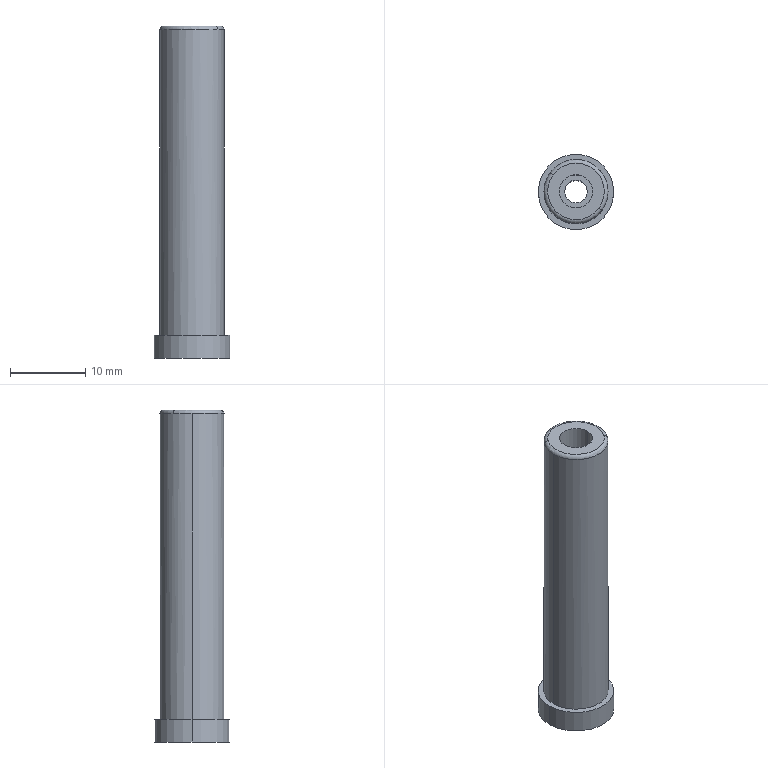Part | 1 solid | 14 faces | box 10 x 10 x 44 mm | volume 2208 mm3 | cylinder 8 | plane 4 | torus 2 | commonest cylinder face diameters 3 x2 4.4 x2 8.5 x2 10 x2
STEP:
#1=CARTESIAN_POINT('',(0.,0.,0.));
#2=DIRECTION('',(0.,0.,1.));
#3=DIRECTION('',(1.,0.,0.));
#4=AXIS2_PLACEMENT_3D('',#1,#2,#3);
#5=CARTESIAN_POINT('',(-237.064,494.704,-190.601));
#6=VERTEX_POINT('',#5);
#7=CARTESIAN_POINT('',(-243.132,494.704,-190.601));
#8=VERTEX_POINT('',#7);
#9=CARTESIAN_POINT('',(-240.098,492.5,-190.601));
#10=DIRECTION('',(0.,0.,1.));
#11=DIRECTION('',(0.809,0.5878,0.));
#12=AXIS2_PLACEMENT_3D('',#9,#10,#11);
#13=CIRCLE('',#12,3.75);
#14=CARTESIAN_POINT('',(-240.098,492.5,-190.601));
#15=DIRECTION('',(0.,0.,1.));
#16=DIRECTION('',(-1.,0.,0.));
#17=AXIS2_PLACEMENT_3D('',#14,#15,#16);
#18=PLANE('',#17);
#19=CARTESIAN_POINT('',(0.,0.));
#20=DIRECTION('',(-0.809,-0.5878));
#21=AXIS2_PLACEMENT_2D('',#19,#20);
#22=CIRCLE('',#21,3.75);
#23=(GEOMETRIC_REPRESENTATION_CONTEXT(2)PARAMETRIC_REPRESENTATION_CONTEXT()REPRESENTATION_CONTEXT('',''));
#24=DEFINITIONAL_REPRESENTATION('',(#22),#23);
#25=PCURVE('',#18,#24);
#26=CARTESIAN_POINT('',(-240.098,492.5,-191.101));
#27=DIRECTION('',(0.,0.,1.));
#28=DIRECTION('',(-0.5878,-0.809,0.));
#29=AXIS2_PLACEMENT_3D('',#26,#27,#28);
#30=TOROIDAL_SURFACE('',#29,3.75,0.5);
#31=CARTESIAN_POINT('',(2.827,1.571));
#32=DIRECTION('',(1.,0.));
#33=VECTOR('',#32,1.);
#34=LINE('',#31,#33);
#35=(GEOMETRIC_REPRESENTATION_CONTEXT(2)PARAMETRIC_REPRESENTATION_CONTEXT()REPRESENTATION_CONTEXT('',''));
#36=DEFINITIONAL_REPRESENTATION('',(#34),#35);
#37=PCURVE('',#30,#36);
#38=SURFACE_CURVE('',#13,(#25,#37),.PCURVE_S1.);
#39=EDGE_CURVE('',#6,#8,#38,.T.);
#40=ORIENTED_EDGE('',*,*,#39,.T.);
#41=CARTESIAN_POINT('',(-237.064,490.296,-190.601));
#42=VERTEX_POINT('',#41);
#43=CARTESIAN_POINT('',(-240.098,492.5,-190.601));
#44=DIRECTION('',(0.,0.,1.));
#45=DIRECTION('',(0.809,0.5878,0.));
#46=AXIS2_PLACEMENT_3D('',#43,#44,#45);
#47=CIRCLE('',#46,3.75);
#48=CARTESIAN_POINT('',(0.,0.));
#49=DIRECTION('',(-0.809,-0.5878));
#50=AXIS2_PLACEMENT_2D('',#48,#49);
#51=CIRCLE('',#50,3.75);
#52=(GEOMETRIC_REPRESENTATION_CONTEXT(2)PARAMETRIC_REPRESENTATION_CONTEXT()REPRESENTATION_CONTEXT('',''));
#53=DEFINITIONAL_REPRESENTATION('',(#51),#52);
#54=PCURVE('',#18,#53);
#55=CARTESIAN_POINT('',(-240.098,492.5,-191.101));
#56=DIRECTION('',(0.,0.,1.));
#57=DIRECTION('',(0.5878,0.809,0.));
#58=AXIS2_PLACEMENT_3D('',#55,#56,#57);
#59=TOROIDAL_SURFACE('',#58,3.75,0.5);
#60=CARTESIAN_POINT('',(-0.3142,1.571));
#61=DIRECTION('',(1.,0.));
#62=VECTOR('',#61,1.);
#63=LINE('',#60,#62);
#64=(GEOMETRIC_REPRESENTATION_CONTEXT(2)PARAMETRIC_REPRESENTATION_CONTEXT()REPRESENTATION_CONTEXT('',''));
#65=DEFINITIONAL_REPRESENTATION('',(#63),#64);
#66=PCURVE('',#59,#65);
#67=SURFACE_CURVE('',#47,(#54,#66),.PCURVE_S1.);
#68=EDGE_CURVE('',#8,#42,#67,.T.);
#69=ORIENTED_EDGE('',*,*,#68,.T.);
#70=CARTESIAN_POINT('',(-240.098,492.5,-190.601));
#71=DIRECTION('',(0.,0.,1.));
#72=DIRECTION('',(0.809,0.5878,0.));
#73=AXIS2_PLACEMENT_3D('',#70,#71,#72);
#74=CIRCLE('',#73,3.75);
#75=CARTESIAN_POINT('',(0.,0.));
#76=DIRECTION('',(-0.809,-0.5878));
#77=AXIS2_PLACEMENT_2D('',#75,#76);
#78=CIRCLE('',#77,3.75);
#79=(GEOMETRIC_REPRESENTATION_CONTEXT(2)PARAMETRIC_REPRESENTATION_CONTEXT()REPRESENTATION_CONTEXT('',''));
#80=DEFINITIONAL_REPRESENTATION('',(#78),#79);
#81=PCURVE('',#18,#80);
#82=CARTESIAN_POINT('',(-3.456,1.571));
#83=DIRECTION('',(1.,0.));
#84=VECTOR('',#83,1.);
#85=LINE('',#82,#84);
#86=(GEOMETRIC_REPRESENTATION_CONTEXT(2)PARAMETRIC_REPRESENTATION_CONTEXT()REPRESENTATION_CONTEXT('',''));
#87=DEFINITIONAL_REPRESENTATION('',(#85),#86);
#88=PCURVE('',#30,#87);
#89=SURFACE_CURVE('',#74,(#81,#88),.PCURVE_S1.);
#90=EDGE_CURVE('',#42,#6,#89,.T.);
#91=ORIENTED_EDGE('',*,*,#90,.T.);
#92=EDGE_LOOP('',(#40,#69,#91));
#93=FACE_BOUND('',#92,.T.);
#94=CARTESIAN_POINT('',(-242.298,492.5,-190.601));
#95=VERTEX_POINT('',#94);
#96=CARTESIAN_POINT('',(-237.898,492.5,-190.601));
#97=VERTEX_POINT('',#96);
#98=CARTESIAN_POINT('',(-240.098,492.5,-190.601));
#99=DIRECTION('',(0.,0.,-1.));
#100=DIRECTION('',(-1.,0.,0.));
#101=AXIS2_PLACEMENT_3D('',#98,#99,#100);
#102=CIRCLE('',#101,2.2);
#103=CARTESIAN_POINT('',(2.2,0.));
#104=CARTESIAN_POINT('',(2.2,-3.811));
#105=CARTESIAN_POINT('',(-1.1,-1.905));
#106=CARTESIAN_POINT('',(-4.4,0.));
#107=CARTESIAN_POINT('',(-1.1,1.905));
#108=CARTESIAN_POINT('',(2.2,3.811));
#109=CARTESIAN_POINT('',(2.2,0.));
#110=(BOUNDED_CURVE()B_SPLINE_CURVE(2,(#103,#104,#105,#106,#107,#108,#109),.UNSPECIFIED.,.T.,.F.)B_SPLINE_CURVE_WITH_KNOTS((1,2,2,2,2,1),(-2.094,0.,2.094,4.189,6.283,8.378),.UNSPECIFIED.)CURVE()GEOMETRIC_REPRESENTATION_ITEM()RATIONAL_B_SPLINE_CURVE((1.,0.5,1.,0.5,1.,0.5,1.))REPRESENTATION_ITEM(''));
#111=(GEOMETRIC_REPRESENTATION_CONTEXT(2)PARAMETRIC_REPRESENTATION_CONTEXT()REPRESENTATION_CONTEXT('',''));
#112=DEFINITIONAL_REPRESENTATION('',(#110),#111);
#113=PCURVE('',#18,#112);
#114=CARTESIAN_POINT('',(-240.098,492.5,-195.701));
#115=DIRECTION('',(0.,0.,1.));
#116=DIRECTION('',(0.,-1.,0.));
#117=AXIS2_PLACEMENT_3D('',#114,#115,#116);
#118=CYLINDRICAL_SURFACE('',#117,2.2);
#119=CARTESIAN_POINT('',(4.712,5.1));
#120=DIRECTION('',(-1.,0.));
#121=VECTOR('',#120,1.);
#122=LINE('',#119,#121);
#123=(GEOMETRIC_REPRESENTATION_CONTEXT(2)PARAMETRIC_REPRESENTATION_CONTEXT()REPRESENTATION_CONTEXT('',''));
#124=DEFINITIONAL_REPRESENTATION('',(#122),#123);
#125=PCURVE('',#118,#124);
#126=SURFACE_CURVE('',#102,(#113,#125),.PCURVE_S1.);
#127=EDGE_CURVE('',#95,#97,#126,.T.);
#128=ORIENTED_EDGE('',*,*,#127,.T.);
#129=CARTESIAN_POINT('',(-240.098,492.5,-190.601));
#130=DIRECTION('',(0.,0.,-1.));
#131=DIRECTION('',(-1.,0.,0.));
#132=AXIS2_PLACEMENT_3D('',#129,#130,#131);
#133=CIRCLE('',#132,2.2);
#134=CARTESIAN_POINT('',(2.2,0.));
#135=CARTESIAN_POINT('',(2.2,-3.811));
#136=CARTESIAN_POINT('',(-1.1,-1.905));
#137=CARTESIAN_POINT('',(-4.4,0.));
#138=CARTESIAN_POINT('',(-1.1,1.905));
#139=CARTESIAN_POINT('',(2.2,3.811));
#140=CARTESIAN_POINT('',(2.2,0.));
#141=(BOUNDED_CURVE()B_SPLINE_CURVE(2,(#134,#135,#136,#137,#138,#139,#140),.UNSPECIFIED.,.T.,.F.)B_SPLINE_CURVE_WITH_KNOTS((1,2,2,2,2,1),(-2.094,0.,2.094,4.189,6.283,8.378),.UNSPECIFIED.)CURVE()GEOMETRIC_REPRESENTATION_ITEM()RATIONAL_B_SPLINE_CURVE((1.,0.5,1.,0.5,1.,0.5,1.))REPRESENTATION_ITEM(''));
#142=(GEOMETRIC_REPRESENTATION_CONTEXT(2)PARAMETRIC_REPRESENTATION_CONTEXT()REPRESENTATION_CONTEXT('',''));
#143=DEFINITIONAL_REPRESENTATION('',(#141),#142);
#144=PCURVE('',#18,#143);
#145=CARTESIAN_POINT('',(-240.098,492.5,-195.701));
#146=DIRECTION('',(0.,0.,1.));
#147=DIRECTION('',(0.,1.,0.));
#148=AXIS2_PLACEMENT_3D('',#145,#146,#147);
#149=CYLINDRICAL_SURFACE('',#148,2.2);
#150=CARTESIAN_POINT('',(7.854,5.1));
#151=DIRECTION('',(-1.,0.));
#152=VECTOR('',#151,1.);
#153=LINE('',#150,#152);
#154=(GEOMETRIC_REPRESENTATION_CONTEXT(2)PARAMETRIC_REPRESENTATION_CONTEXT()REPRESENTATION_CONTEXT('',''));
#155=DEFINITIONAL_REPRESENTATION('',(#153),#154);
#156=PCURVE('',#149,#155);
#157=SURFACE_CURVE('',#133,(#144,#156),.PCURVE_S1.);
#158=EDGE_CURVE('',#97,#95,#157,.T.);
#159=ORIENTED_EDGE('',*,*,#158,.T.);
#160=EDGE_LOOP('',(#128,#159));
#161=FACE_BOUND('',#160,.T.);
#162=ADVANCED_FACE('',(#93,#161),#18,.T.);
#163=CARTESIAN_POINT('',(-237.898,492.5,-195.701));
#164=VERTEX_POINT('',#163);
#165=CARTESIAN_POINT('',(-242.298,492.5,-195.701));
#166=VERTEX_POINT('',#165);
#167=CARTESIAN_POINT('',(-240.098,492.5,-195.701));
#168=DIRECTION('',(0.,0.,1.));
#169=DIRECTION('',(-1.,0.,0.));
#170=AXIS2_PLACEMENT_3D('',#167,#168,#169);
#171=CIRCLE('',#170,2.2);
#172=CARTESIAN_POINT('',(-1.571,0.));
#173=DIRECTION('',(1.,0.));
#174=VECTOR('',#173,1.);
#175=LINE('',#172,#174);
#176=(GEOMETRIC_REPRESENTATION_CONTEXT(2)PARAMETRIC_REPRESENTATION_CONTEXT()REPRESENTATION_CONTEXT('',''));
#177=DEFINITIONAL_REPRESENTATION('',(#175),#176);
#178=PCURVE('',#118,#177);
#179=CARTESIAN_POINT('',(-240.098,492.5,-195.701));
#180=DIRECTION('',(0.,0.,-1.));
#181=DIRECTION('',(1.,0.,0.));
#182=AXIS2_PLACEMENT_3D('',#179,#180,#181);
#183=PLANE('',#182);
#184=CARTESIAN_POINT('',(-2.2,0.));
#185=CARTESIAN_POINT('',(-2.2,3.811));
#186=CARTESIAN_POINT('',(1.1,1.905));
#187=CARTESIAN_POINT('',(4.4,0.));
#188=CARTESIAN_POINT('',(1.1,-1.905));
#189=CARTESIAN_POINT('',(-2.2,-3.811));
#190=CARTESIAN_POINT('',(-2.2,0.));
#191=(BOUNDED_CURVE()B_SPLINE_CURVE(2,(#184,#185,#186,#187,#188,#189,#190),.UNSPECIFIED.,.T.,.F.)B_SPLINE_CURVE_WITH_KNOTS((1,2,2,2,2,1),(-2.094,0.,2.094,4.189,6.283,8.378),.UNSPECIFIED.)CURVE()GEOMETRIC_REPRESENTATION_ITEM()RATIONAL_B_SPLINE_CURVE((1.,0.5,1.,0.5,1.,0.5,1.))REPRESENTATION_ITEM(''));
#192=(GEOMETRIC_REPRESENTATION_CONTEXT(2)PARAMETRIC_REPRESENTATION_CONTEXT()REPRESENTATION_CONTEXT('',''));
#193=DEFINITIONAL_REPRESENTATION('',(#191),#192);
#194=PCURVE('',#183,#193);
#195=SURFACE_CURVE('',#171,(#178,#194),.PCURVE_S1.);
#196=EDGE_CURVE('',#164,#166,#195,.T.);
#197=ORIENTED_EDGE('',*,*,#196,.T.);
#198=CARTESIAN_POINT('',(-242.298,492.5,-195.701));
#199=DIRECTION('',(0.,0.,1.));
#200=VECTOR('',#199,1.);
#201=LINE('',#198,#200);
#202=CARTESIAN_POINT('',(4.712,0.));
#203=DIRECTION('',(0.,1.));
#204=VECTOR('',#203,1.);
#205=LINE('',#202,#204);
#206=(GEOMETRIC_REPRESENTATION_CONTEXT(2)PARAMETRIC_REPRESENTATION_CONTEXT()REPRESENTATION_CONTEXT('',''));
#207=DEFINITIONAL_REPRESENTATION('',(#205),#206);
#208=PCURVE('',#118,#207);
#209=CARTESIAN_POINT('',(1.571,0.));
#210=DIRECTION('',(0.,1.));
#211=VECTOR('',#210,1.);
#212=LINE('',#209,#211);
#213=(GEOMETRIC_REPRESENTATION_CONTEXT(2)PARAMETRIC_REPRESENTATION_CONTEXT()REPRESENTATION_CONTEXT('',''));
#214=DEFINITIONAL_REPRESENTATION('',(#212),#213);
#215=PCURVE('',#149,#214);
#216=SURFACE_CURVE('',#201,(#208,#215),.PCURVE_S1.);
#217=EDGE_CURVE('',#166,#95,#216,.T.);
#218=ORIENTED_EDGE('',*,*,#217,.T.);
#219=ORIENTED_EDGE('',*,*,#127,.T.);
#220=CARTESIAN_POINT('',(-237.898,492.5,-195.701));
#221=DIRECTION('',(0.,0.,1.));
#222=VECTOR('',#221,1.);
#223=LINE('',#220,#222);
#224=CARTESIAN_POINT('',(1.571,0.));
#225=DIRECTION('',(0.,1.));
#226=VECTOR('',#225,1.);
#227=LINE('',#224,#226);
#228=(GEOMETRIC_REPRESENTATION_CONTEXT(2)PARAMETRIC_REPRESENTATION_CONTEXT()REPRESENTATION_CONTEXT('',''));
#229=DEFINITIONAL_REPRESENTATION('',(#227),#228);
#230=PCURVE('',#118,#229);
#231=CARTESIAN_POINT('',(4.712,0.));
#232=DIRECTION('',(0.,1.));
#233=VECTOR('',#232,1.);
#234=LINE('',#231,#233);
#235=(GEOMETRIC_REPRESENTATION_CONTEXT(2)PARAMETRIC_REPRESENTATION_CONTEXT()REPRESENTATION_CONTEXT('',''));
#236=DEFINITIONAL_REPRESENTATION('',(#234),#235);
#237=PCURVE('',#149,#236);
#238=SURFACE_CURVE('',#223,(#230,#237),.PCURVE_S1.);
#239=EDGE_CURVE('',#164,#97,#238,.T.);
#240=ORIENTED_EDGE('',*,*,#239,.F.);
#241=EDGE_LOOP('',(#197,#218,#219,#240));
#242=FACE_BOUND('',#241,.F.);
#243=ADVANCED_FACE('',(#242),#118,.F.);
#244=CARTESIAN_POINT('',(-240.098,492.5,-195.701));
#245=DIRECTION('',(0.,0.,1.));
#246=DIRECTION('',(-1.,0.,0.));
#247=AXIS2_PLACEMENT_3D('',#244,#245,#246);
#248=CIRCLE('',#247,2.2);
#249=CARTESIAN_POINT('',(-2.2,0.));
#250=CARTESIAN_POINT('',(-2.2,3.811));
#251=CARTESIAN_POINT('',(1.1,1.905));
#252=CARTESIAN_POINT('',(4.4,0.));
#253=CARTESIAN_POINT('',(1.1,-1.905));
#254=CARTESIAN_POINT('',(-2.2,-3.811));
#255=CARTESIAN_POINT('',(-2.2,0.));
#256=(BOUNDED_CURVE()B_SPLINE_CURVE(2,(#249,#250,#251,#252,#253,#254,#255),.UNSPECIFIED.,.T.,.F.)B_SPLINE_CURVE_WITH_KNOTS((1,2,2,2,2,1),(-2.094,0.,2.094,4.189,6.283,8.378),.UNSPECIFIED.)CURVE()GEOMETRIC_REPRESENTATION_ITEM()RATIONAL_B_SPLINE_CURVE((1.,0.5,1.,0.5,1.,0.5,1.))REPRESENTATION_ITEM(''));
#257=(GEOMETRIC_REPRESENTATION_CONTEXT(2)PARAMETRIC_REPRESENTATION_CONTEXT()REPRESENTATION_CONTEXT('',''));
#258=DEFINITIONAL_REPRESENTATION('',(#256),#257);
#259=PCURVE('',#183,#258);
#260=CARTESIAN_POINT('',(1.571,0.));
#261=DIRECTION('',(1.,0.));
#262=VECTOR('',#261,1.);
#263=LINE('',#260,#262);
#264=(GEOMETRIC_REPRESENTATION_CONTEXT(2)PARAMETRIC_REPRESENTATION_CONTEXT()REPRESENTATION_CONTEXT('',''));
#265=DEFINITIONAL_REPRESENTATION('',(#263),#264);
#266=PCURVE('',#149,#265);
#267=SURFACE_CURVE('',#248,(#259,#266),.PCURVE_S1.);
#268=EDGE_CURVE('',#166,#164,#267,.T.);
#269=ORIENTED_EDGE('',*,*,#268,.T.);
#270=ORIENTED_EDGE('',*,*,#196,.T.);
#271=EDGE_LOOP('',(#269,#270));
#272=FACE_BOUND('',#271,.T.);
#273=CARTESIAN_POINT('',(-241.598,492.5,-195.701));
#274=VERTEX_POINT('',#273);
#275=CARTESIAN_POINT('',(-238.598,492.5,-195.701));
#276=VERTEX_POINT('',#275);
#277=CARTESIAN_POINT('',(-240.098,492.5,-195.701));
#278=DIRECTION('',(0.,0.,1.));
#279=DIRECTION('',(1.,0.,0.));
#280=AXIS2_PLACEMENT_3D('',#277,#278,#279);
#281=CIRCLE('',#280,1.5);
#282=CARTESIAN_POINT('',(1.5,0.));
#283=CARTESIAN_POINT('',(1.5,-2.598));
#284=CARTESIAN_POINT('',(-0.75,-1.299));
#285=CARTESIAN_POINT('',(-3.,0.));
#286=CARTESIAN_POINT('',(-0.75,1.299));
#287=CARTESIAN_POINT('',(1.5,2.598));
#288=CARTESIAN_POINT('',(1.5,0.));
#289=(BOUNDED_CURVE()B_SPLINE_CURVE(2,(#282,#283,#284,#285,#286,#287,#288),.UNSPECIFIED.,.T.,.F.)B_SPLINE_CURVE_WITH_KNOTS((1,2,2,2,2,1),(-2.094,0.,2.094,4.189,6.283,8.378),.UNSPECIFIED.)CURVE()GEOMETRIC_REPRESENTATION_ITEM()RATIONAL_B_SPLINE_CURVE((1.,0.5,1.,0.5,1.,0.5,1.))REPRESENTATION_ITEM(''));
#290=(GEOMETRIC_REPRESENTATION_CONTEXT(2)PARAMETRIC_REPRESENTATION_CONTEXT()REPRESENTATION_CONTEXT('',''));
#291=DEFINITIONAL_REPRESENTATION('',(#289),#290);
#292=PCURVE('',#183,#291);
#293=CARTESIAN_POINT('',(-240.098,492.5,-190.601));
#294=DIRECTION('',(0.,0.,-1.));
#295=DIRECTION('',(0.,1.,0.));
#296=AXIS2_PLACEMENT_3D('',#293,#294,#295);
#297=CYLINDRICAL_SURFACE('',#296,1.5);
#298=CARTESIAN_POINT('',(7.854,5.1));
#299=DIRECTION('',(-1.,0.));
#300=VECTOR('',#299,1.);
#301=LINE('',#298,#300);
#302=(GEOMETRIC_REPRESENTATION_CONTEXT(2)PARAMETRIC_REPRESENTATION_CONTEXT()REPRESENTATION_CONTEXT('',''));
#303=DEFINITIONAL_REPRESENTATION('',(#301),#302);
#304=PCURVE('',#297,#303);
#305=SURFACE_CURVE('',#281,(#292,#304),.PCURVE_S1.);
#306=EDGE_CURVE('',#274,#276,#305,.T.);
#307=ORIENTED_EDGE('',*,*,#306,.F.);
#308=CARTESIAN_POINT('',(-240.098,492.5,-195.701));
#309=DIRECTION('',(0.,0.,1.));
#310=DIRECTION('',(1.,0.,0.));
#311=AXIS2_PLACEMENT_3D('',#308,#309,#310);
#312=CIRCLE('',#311,1.5);
#313=CARTESIAN_POINT('',(1.5,0.));
#314=CARTESIAN_POINT('',(1.5,-2.598));
#315=CARTESIAN_POINT('',(-0.75,-1.299));
#316=CARTESIAN_POINT('',(-3.,0.));
#317=CARTESIAN_POINT('',(-0.75,1.299));
#318=CARTESIAN_POINT('',(1.5,2.598));
#319=CARTESIAN_POINT('',(1.5,0.));
#320=(BOUNDED_CURVE()B_SPLINE_CURVE(2,(#313,#314,#315,#316,#317,#318,#319),.UNSPECIFIED.,.T.,.F.)B_SPLINE_CURVE_WITH_KNOTS((1,2,2,2,2,1),(-2.094,0.,2.094,4.189,6.283,8.378),.UNSPECIFIED.)CURVE()GEOMETRIC_REPRESENTATION_ITEM()RATIONAL_B_SPLINE_CURVE((1.,0.5,1.,0.5,1.,0.5,1.))REPRESENTATION_ITEM(''));
#321=(GEOMETRIC_REPRESENTATION_CONTEXT(2)PARAMETRIC_REPRESENTATION_CONTEXT()REPRESENTATION_CONTEXT('',''));
#322=DEFINITIONAL_REPRESENTATION('',(#320),#321);
#323=PCURVE('',#183,#322);
#324=CARTESIAN_POINT('',(-240.098,492.5,-190.601));
#325=DIRECTION('',(0.,0.,-1.));
#326=DIRECTION('',(0.,-1.,0.));
#327=AXIS2_PLACEMENT_3D('',#324,#325,#326);
#328=CYLINDRICAL_SURFACE('',#327,1.5);
#329=CARTESIAN_POINT('',(4.712,5.1));
#330=DIRECTION('',(-1.,0.));
#331=VECTOR('',#330,1.);
#332=LINE('',#329,#331);
#333=(GEOMETRIC_REPRESENTATION_CONTEXT(2)PARAMETRIC_REPRESENTATION_CONTEXT()REPRESENTATION_CONTEXT('',''));
#334=DEFINITIONAL_REPRESENTATION('',(#332),#333);
#335=PCURVE('',#328,#334);
#336=SURFACE_CURVE('',#312,(#323,#335),.PCURVE_S1.);
#337=EDGE_CURVE('',#276,#274,#336,.T.);
#338=ORIENTED_EDGE('',*,*,#337,.F.);
#339=EDGE_LOOP('',(#307,#338));
#340=FACE_BOUND('',#339,.T.);
#341=ADVANCED_FACE('',(#272,#340),#183,.F.);
#342=ORIENTED_EDGE('',*,*,#337,.F.);
#343=CARTESIAN_POINT('',(-238.598,492.5,-234.601));
#344=VERTEX_POINT('',#343);
#345=CARTESIAN_POINT('',(-238.598,492.5,-195.701));
#346=DIRECTION('',(0.,0.,-1.));
#347=VECTOR('',#346,1.);
#348=LINE('',#345,#347);
#349=CARTESIAN_POINT('',(4.712,5.1));
#350=DIRECTION('',(0.,1.));
#351=VECTOR('',#350,1.);
#352=LINE('',#349,#351);
#353=(GEOMETRIC_REPRESENTATION_CONTEXT(2)PARAMETRIC_REPRESENTATION_CONTEXT()REPRESENTATION_CONTEXT('',''));
#354=DEFINITIONAL_REPRESENTATION('',(#352),#353);
#355=PCURVE('',#328,#354);
#356=CARTESIAN_POINT('',(1.571,5.1));
#357=DIRECTION('',(0.,1.));
#358=VECTOR('',#357,1.);
#359=LINE('',#356,#358);
#360=(GEOMETRIC_REPRESENTATION_CONTEXT(2)PARAMETRIC_REPRESENTATION_CONTEXT()REPRESENTATION_CONTEXT('',''));
#361=DEFINITIONAL_REPRESENTATION('',(#359),#360);
#362=PCURVE('',#297,#361);
#363=SURFACE_CURVE('',#348,(#355,#362),.PCURVE_S1.);
#364=EDGE_CURVE('',#276,#344,#363,.T.);
#365=ORIENTED_EDGE('',*,*,#364,.T.);
#366=CARTESIAN_POINT('',(-241.598,492.5,-234.601));
#367=VERTEX_POINT('',#366);
#368=CARTESIAN_POINT('',(-240.098,492.5,-234.601));
#369=DIRECTION('',(0.,0.,-1.));
#370=DIRECTION('',(1.,0.,0.));
#371=AXIS2_PLACEMENT_3D('',#368,#369,#370);
#372=CIRCLE('',#371,1.5);
#373=CARTESIAN_POINT('',(-1.571,44.));
#374=DIRECTION('',(1.,0.));
#375=VECTOR('',#374,1.);
#376=LINE('',#373,#375);
#377=(GEOMETRIC_REPRESENTATION_CONTEXT(2)PARAMETRIC_REPRESENTATION_CONTEXT()REPRESENTATION_CONTEXT('',''));
#378=DEFINITIONAL_REPRESENTATION('',(#376),#377);
#379=PCURVE('',#328,#378);
#380=CARTESIAN_POINT('',(-240.098,492.5,-234.601));
#381=DIRECTION('',(0.,0.,-1.));
#382=DIRECTION('',(1.,0.,0.));
#383=AXIS2_PLACEMENT_3D('',#380,#381,#382);
#384=PLANE('',#383);
#385=CARTESIAN_POINT('',(0.,0.));
#386=DIRECTION('',(1.,0.));
#387=AXIS2_PLACEMENT_2D('',#385,#386);
#388=CIRCLE('',#387,1.5);
#389=(GEOMETRIC_REPRESENTATION_CONTEXT(2)PARAMETRIC_REPRESENTATION_CONTEXT()REPRESENTATION_CONTEXT('',''));
#390=DEFINITIONAL_REPRESENTATION('',(#388),#389);
#391=PCURVE('',#384,#390);
#392=SURFACE_CURVE('',#372,(#379,#391),.PCURVE_S1.);
#393=EDGE_CURVE('',#367,#344,#392,.T.);
#394=ORIENTED_EDGE('',*,*,#393,.F.);
#395=CARTESIAN_POINT('',(-241.598,492.5,-195.701));
#396=DIRECTION('',(0.,0.,-1.));
#397=VECTOR('',#396,1.);
#398=LINE('',#395,#397);
#399=CARTESIAN_POINT('',(1.571,5.1));
#400=DIRECTION('',(0.,1.));
#401=VECTOR('',#400,1.);
#402=LINE('',#399,#401);
#403=(GEOMETRIC_REPRESENTATION_CONTEXT(2)PARAMETRIC_REPRESENTATION_CONTEXT()REPRESENTATION_CONTEXT('',''));
#404=DEFINITIONAL_REPRESENTATION('',(#402),#403);
#405=PCURVE('',#328,#404);
#406=CARTESIAN_POINT('',(4.712,5.1));
#407=DIRECTION('',(0.,1.));
#408=VECTOR('',#407,1.);
#409=LINE('',#406,#408);
#410=(GEOMETRIC_REPRESENTATION_CONTEXT(2)PARAMETRIC_REPRESENTATION_CONTEXT()REPRESENTATION_CONTEXT('',''));
#411=DEFINITIONAL_REPRESENTATION('',(#409),#410);
#412=PCURVE('',#297,#411);
#413=SURFACE_CURVE('',#398,(#405,#412),.PCURVE_S1.);
#414=EDGE_CURVE('',#274,#367,#413,.T.);
#415=ORIENTED_EDGE('',*,*,#414,.F.);
#416=EDGE_LOOP('',(#342,#365,#394,#415));
#417=FACE_BOUND('',#416,.F.);
#418=ADVANCED_FACE('',(#417),#328,.F.);
#419=ORIENTED_EDGE('',*,*,#393,.F.);
#420=CARTESIAN_POINT('',(-240.098,492.5,-234.601));
#421=DIRECTION('',(0.,0.,-1.));
#422=DIRECTION('',(1.,0.,0.));
#423=AXIS2_PLACEMENT_3D('',#420,#421,#422);
#424=CIRCLE('',#423,1.5);
#425=CARTESIAN_POINT('',(0.,0.));
#426=DIRECTION('',(1.,0.));
#427=AXIS2_PLACEMENT_2D('',#425,#426);
#428=CIRCLE('',#427,1.5);
#429=(GEOMETRIC_REPRESENTATION_CONTEXT(2)PARAMETRIC_REPRESENTATION_CONTEXT()REPRESENTATION_CONTEXT('',''));
#430=DEFINITIONAL_REPRESENTATION('',(#428),#429);
#431=PCURVE('',#384,#430);
#432=CARTESIAN_POINT('',(1.571,44.));
#433=DIRECTION('',(1.,0.));
#434=VECTOR('',#433,1.);
#435=LINE('',#432,#434);
#436=(GEOMETRIC_REPRESENTATION_CONTEXT(2)PARAMETRIC_REPRESENTATION_CONTEXT()REPRESENTATION_CONTEXT('',''));
#437=DEFINITIONAL_REPRESENTATION('',(#435),#436);
#438=PCURVE('',#297,#437);
#439=SURFACE_CURVE('',#424,(#431,#438),.PCURVE_S1.);
#440=EDGE_CURVE('',#344,#367,#439,.T.);
#441=ORIENTED_EDGE('',*,*,#440,.F.);
#442=EDGE_LOOP('',(#419,#441));
#443=FACE_BOUND('',#442,.T.);
#444=CARTESIAN_POINT('',(-245.098,492.5,-234.601));
#445=VERTEX_POINT('',#444);
#446=CARTESIAN_POINT('',(-235.098,492.5,-234.601));
#447=VERTEX_POINT('',#446);
#448=CARTESIAN_POINT('',(-240.098,492.5,-234.601));
#449=DIRECTION('',(0.,0.,-1.));
#450=DIRECTION('',(-1.,0.,0.));
#451=AXIS2_PLACEMENT_3D('',#448,#449,#450);
#452=CIRCLE('',#451,5.);
#453=CARTESIAN_POINT('',(0.,0.));
#454=DIRECTION('',(-1.,0.));
#455=AXIS2_PLACEMENT_2D('',#453,#454);
#456=CIRCLE('',#455,5.);
#457=(GEOMETRIC_REPRESENTATION_CONTEXT(2)PARAMETRIC_REPRESENTATION_CONTEXT()REPRESENTATION_CONTEXT('',''));
#458=DEFINITIONAL_REPRESENTATION('',(#456),#457);
#459=PCURVE('',#384,#458);
#460=CARTESIAN_POINT('',(-240.098,492.5,-234.601));
#461=DIRECTION('',(0.,0.,1.));
#462=DIRECTION('',(0.,-1.,0.));
#463=AXIS2_PLACEMENT_3D('',#460,#461,#462);
#464=CYLINDRICAL_SURFACE('',#463,5.);
#465=CARTESIAN_POINT('',(4.712,0.));
#466=DIRECTION('',(-1.,0.));
#467=VECTOR('',#466,1.);
#468=LINE('',#465,#467);
#469=(GEOMETRIC_REPRESENTATION_CONTEXT(2)PARAMETRIC_REPRESENTATION_CONTEXT()REPRESENTATION_CONTEXT('',''));
#470=DEFINITIONAL_REPRESENTATION('',(#468),#469);
#471=PCURVE('',#464,#470);
#472=SURFACE_CURVE('',#452,(#459,#471),.PCURVE_S1.);
#473=EDGE_CURVE('',#445,#447,#472,.T.);
#474=ORIENTED_EDGE('',*,*,#473,.T.);
#475=CARTESIAN_POINT('',(-240.098,492.5,-234.601));
#476=DIRECTION('',(0.,0.,-1.));
#477=DIRECTION('',(-1.,0.,0.));
#478=AXIS2_PLACEMENT_3D('',#475,#476,#477);
#479=CIRCLE('',#478,5.);
#480=CARTESIAN_POINT('',(0.,0.));
#481=DIRECTION('',(-1.,0.));
#482=AXIS2_PLACEMENT_2D('',#480,#481);
#483=CIRCLE('',#482,5.);
#484=(GEOMETRIC_REPRESENTATION_CONTEXT(2)PARAMETRIC_REPRESENTATION_CONTEXT()REPRESENTATION_CONTEXT('',''));
#485=DEFINITIONAL_REPRESENTATION('',(#483),#484);
#486=PCURVE('',#384,#485);
#487=CARTESIAN_POINT('',(-240.098,492.5,-234.601));
#488=DIRECTION('',(0.,0.,1.));
#489=DIRECTION('',(0.,1.,0.));
#490=AXIS2_PLACEMENT_3D('',#487,#488,#489);
#491=CYLINDRICAL_SURFACE('',#490,5.);
#492=CARTESIAN_POINT('',(7.854,0.));
#493=DIRECTION('',(-1.,0.));
#494=VECTOR('',#493,1.);
#495=LINE('',#492,#494);
#496=(GEOMETRIC_REPRESENTATION_CONTEXT(2)PARAMETRIC_REPRESENTATION_CONTEXT()REPRESENTATION_CONTEXT('',''));
#497=DEFINITIONAL_REPRESENTATION('',(#495),#496);
#498=PCURVE('',#491,#497);
#499=SURFACE_CURVE('',#479,(#486,#498),.PCURVE_S1.);
#500=EDGE_CURVE('',#447,#445,#499,.T.);
#501=ORIENTED_EDGE('',*,*,#500,.T.);
#502=EDGE_LOOP('',(#474,#501));
#503=FACE_BOUND('',#502,.T.);
#504=ADVANCED_FACE('',(#443,#503),#384,.T.);
#505=CARTESIAN_POINT('',(-235.098,492.5,-231.601));
#506=VERTEX_POINT('',#505);
#507=CARTESIAN_POINT('',(-235.098,492.5,-234.601));
#508=DIRECTION('',(0.,0.,1.));
#509=VECTOR('',#508,1.);
#510=LINE('',#507,#509);
#511=CARTESIAN_POINT('',(1.571,0.));
#512=DIRECTION('',(0.,1.));
#513=VECTOR('',#512,1.);
#514=LINE('',#511,#513);
#515=(GEOMETRIC_REPRESENTATION_CONTEXT(2)PARAMETRIC_REPRESENTATION_CONTEXT()REPRESENTATION_CONTEXT('',''));
#516=DEFINITIONAL_REPRESENTATION('',(#514),#515);
#517=PCURVE('',#464,#516);
#518=CARTESIAN_POINT('',(4.712,0.));
#519=DIRECTION('',(0.,1.));
#520=VECTOR('',#519,1.);
#521=LINE('',#518,#520);
#522=(GEOMETRIC_REPRESENTATION_CONTEXT(2)PARAMETRIC_REPRESENTATION_CONTEXT()REPRESENTATION_CONTEXT('',''));
#523=DEFINITIONAL_REPRESENTATION('',(#521),#522);
#524=PCURVE('',#491,#523);
#525=SURFACE_CURVE('',#510,(#517,#524),.PCURVE_S1.);
#526=EDGE_CURVE('',#447,#506,#525,.T.);
#527=ORIENTED_EDGE('',*,*,#526,.F.);
#528=ORIENTED_EDGE('',*,*,#473,.F.);
#529=CARTESIAN_POINT('',(-245.098,492.5,-231.601));
#530=VERTEX_POINT('',#529);
#531=CARTESIAN_POINT('',(-245.098,492.5,-234.601));
#532=DIRECTION('',(0.,0.,1.));
#533=VECTOR('',#532,1.);
#534=LINE('',#531,#533);
#535=CARTESIAN_POINT('',(4.712,0.));
#536=DIRECTION('',(0.,1.));
#537=VECTOR('',#536,1.);
#538=LINE('',#535,#537);
#539=(GEOMETRIC_REPRESENTATION_CONTEXT(2)PARAMETRIC_REPRESENTATION_CONTEXT()REPRESENTATION_CONTEXT('',''));
#540=DEFINITIONAL_REPRESENTATION('',(#538),#539);
#541=PCURVE('',#464,#540);
#542=CARTESIAN_POINT('',(1.571,0.));
#543=DIRECTION('',(0.,1.));
#544=VECTOR('',#543,1.);
#545=LINE('',#542,#544);
#546=(GEOMETRIC_REPRESENTATION_CONTEXT(2)PARAMETRIC_REPRESENTATION_CONTEXT()REPRESENTATION_CONTEXT('',''));
#547=DEFINITIONAL_REPRESENTATION('',(#545),#546);
#548=PCURVE('',#491,#547);
#549=SURFACE_CURVE('',#534,(#541,#548),.PCURVE_S1.);
#550=EDGE_CURVE('',#445,#530,#549,.T.);
#551=ORIENTED_EDGE('',*,*,#550,.T.);
#552=CARTESIAN_POINT('',(-240.098,492.5,-231.601));
#553=DIRECTION('',(0.,0.,-1.));
#554=DIRECTION('',(-1.,0.,0.));
#555=AXIS2_PLACEMENT_3D('',#552,#553,#554);
#556=CIRCLE('',#555,5.);
#557=CARTESIAN_POINT('',(4.712,3.));
#558=DIRECTION('',(-1.,0.));
#559=VECTOR('',#558,1.);
#560=LINE('',#557,#559);
#561=(GEOMETRIC_REPRESENTATION_CONTEXT(2)PARAMETRIC_REPRESENTATION_CONTEXT()REPRESENTATION_CONTEXT('',''));
#562=DEFINITIONAL_REPRESENTATION('',(#560),#561);
#563=PCURVE('',#464,#562);
#564=CARTESIAN_POINT('',(-240.098,492.5,-231.601));
#565=DIRECTION('',(0.,0.,-1.));
#566=DIRECTION('',(1.,0.,0.));
#567=AXIS2_PLACEMENT_3D('',#564,#565,#566);
#568=PLANE('',#567);
#569=CARTESIAN_POINT('',(0.,0.));
#570=DIRECTION('',(-1.,0.));
#571=AXIS2_PLACEMENT_2D('',#569,#570);
#572=CIRCLE('',#571,5.);
#573=(GEOMETRIC_REPRESENTATION_CONTEXT(2)PARAMETRIC_REPRESENTATION_CONTEXT()REPRESENTATION_CONTEXT('',''));
#574=DEFINITIONAL_REPRESENTATION('',(#572),#573);
#575=PCURVE('',#568,#574);
#576=SURFACE_CURVE('',#556,(#563,#575),.PCURVE_S1.);
#577=EDGE_CURVE('',#530,#506,#576,.T.);
#578=ORIENTED_EDGE('',*,*,#577,.T.);
#579=EDGE_LOOP('',(#527,#528,#551,#578));
#580=FACE_BOUND('',#579,.T.);
#581=ADVANCED_FACE('',(#580),#464,.T.);
#582=CARTESIAN_POINT('',(-235.848,492.5,-231.601));
#583=VERTEX_POINT('',#582);
#584=CARTESIAN_POINT('',(-244.348,492.5,-231.601));
#585=VERTEX_POINT('',#584);
#586=CARTESIAN_POINT('',(-240.098,492.5,-231.601));
#587=DIRECTION('',(0.,0.,1.));
#588=DIRECTION('',(-1.,0.,0.));
#589=AXIS2_PLACEMENT_3D('',#586,#587,#588);
#590=CIRCLE('',#589,4.25);
#591=CARTESIAN_POINT('',(-4.25,0.));
#592=CARTESIAN_POINT('',(-4.25,7.361));
#593=CARTESIAN_POINT('',(2.125,3.681));
#594=CARTESIAN_POINT('',(8.5,0.));
#595=CARTESIAN_POINT('',(2.125,-3.681));
#596=CARTESIAN_POINT('',(-4.25,-7.361));
#597=CARTESIAN_POINT('',(-4.25,0.));
#598=(BOUNDED_CURVE()B_SPLINE_CURVE(2,(#591,#592,#593,#594,#595,#596,#597),.UNSPECIFIED.,.T.,.F.)B_SPLINE_CURVE_WITH_KNOTS((1,2,2,2,2,1),(-2.094,0.,2.094,4.189,6.283,8.378),.UNSPECIFIED.)CURVE()GEOMETRIC_REPRESENTATION_ITEM()RATIONAL_B_SPLINE_CURVE((1.,0.5,1.,0.5,1.,0.5,1.))REPRESENTATION_ITEM(''));
#599=(GEOMETRIC_REPRESENTATION_CONTEXT(2)PARAMETRIC_REPRESENTATION_CONTEXT()REPRESENTATION_CONTEXT('',''));
#600=DEFINITIONAL_REPRESENTATION('',(#598),#599);
#601=PCURVE('',#568,#600);
#602=CARTESIAN_POINT('',(-240.098,492.5,-231.601));
#603=DIRECTION('',(0.,0.,1.));
#604=DIRECTION('',(0.,-1.,0.));
#605=AXIS2_PLACEMENT_3D('',#602,#603,#604);
#606=CYLINDRICAL_SURFACE('',#605,4.25);
#607=CARTESIAN_POINT('',(-1.571,0.));
#608=DIRECTION('',(1.,0.));
#609=VECTOR('',#608,1.);
#610=LINE('',#607,#609);
#611=(GEOMETRIC_REPRESENTATION_CONTEXT(2)PARAMETRIC_REPRESENTATION_CONTEXT()REPRESENTATION_CONTEXT('',''));
#612=DEFINITIONAL_REPRESENTATION('',(#610),#611);
#613=PCURVE('',#606,#612);
#614=SURFACE_CURVE('',#590,(#601,#613),.PCURVE_S1.);
#615=EDGE_CURVE('',#583,#585,#614,.T.);
#616=ORIENTED_EDGE('',*,*,#615,.F.);
#617=CARTESIAN_POINT('',(-240.098,492.5,-231.601));
#618=DIRECTION('',(0.,0.,1.));
#619=DIRECTION('',(-1.,0.,0.));
#620=AXIS2_PLACEMENT_3D('',#617,#618,#619);
#621=CIRCLE('',#620,4.25);
#622=CARTESIAN_POINT('',(-4.25,0.));
#623=CARTESIAN_POINT('',(-4.25,7.361));
#624=CARTESIAN_POINT('',(2.125,3.681));
#625=CARTESIAN_POINT('',(8.5,0.));
#626=CARTESIAN_POINT('',(2.125,-3.681));
#627=CARTESIAN_POINT('',(-4.25,-7.361));
#628=CARTESIAN_POINT('',(-4.25,0.));
#629=(BOUNDED_CURVE()B_SPLINE_CURVE(2,(#622,#623,#624,#625,#626,#627,#628),.UNSPECIFIED.,.T.,.F.)B_SPLINE_CURVE_WITH_KNOTS((1,2,2,2,2,1),(-2.094,0.,2.094,4.189,6.283,8.378),.UNSPECIFIED.)CURVE()GEOMETRIC_REPRESENTATION_ITEM()RATIONAL_B_SPLINE_CURVE((1.,0.5,1.,0.5,1.,0.5,1.))REPRESENTATION_ITEM(''));
#630=(GEOMETRIC_REPRESENTATION_CONTEXT(2)PARAMETRIC_REPRESENTATION_CONTEXT()REPRESENTATION_CONTEXT('',''));
#631=DEFINITIONAL_REPRESENTATION('',(#629),#630);
#632=PCURVE('',#568,#631);
#633=CARTESIAN_POINT('',(-240.098,492.5,-231.601));
#634=DIRECTION('',(0.,0.,1.));
#635=DIRECTION('',(0.,1.,0.));
#636=AXIS2_PLACEMENT_3D('',#633,#634,#635);
#637=CYLINDRICAL_SURFACE('',#636,4.25);
#638=CARTESIAN_POINT('',(1.571,0.));
#639=DIRECTION('',(1.,0.));
#640=VECTOR('',#639,1.);
#641=LINE('',#638,#640);
#642=(GEOMETRIC_REPRESENTATION_CONTEXT(2)PARAMETRIC_REPRESENTATION_CONTEXT()REPRESENTATION_CONTEXT('',''));
#643=DEFINITIONAL_REPRESENTATION('',(#641),#642);
#644=PCURVE('',#637,#643);
#645=SURFACE_CURVE('',#621,(#632,#644),.PCURVE_S1.);
#646=EDGE_CURVE('',#585,#583,#645,.T.);
#647=ORIENTED_EDGE('',*,*,#646,.F.);
#648=EDGE_LOOP('',(#616,#647));
#649=FACE_BOUND('',#648,.T.);
#650=CARTESIAN_POINT('',(-240.098,492.5,-231.601));
#651=DIRECTION('',(0.,0.,-1.));
#652=DIRECTION('',(-1.,0.,0.));
#653=AXIS2_PLACEMENT_3D('',#650,#651,#652);
#654=CIRCLE('',#653,5.);
#655=CARTESIAN_POINT('',(0.,0.));
#656=DIRECTION('',(-1.,0.));
#657=AXIS2_PLACEMENT_2D('',#655,#656);
#658=CIRCLE('',#657,5.);
#659=(GEOMETRIC_REPRESENTATION_CONTEXT(2)PARAMETRIC_REPRESENTATION_CONTEXT()REPRESENTATION_CONTEXT('',''));
#660=DEFINITIONAL_REPRESENTATION('',(#658),#659);
#661=PCURVE('',#568,#660);
#662=CARTESIAN_POINT('',(7.854,3.));
#663=DIRECTION('',(-1.,0.));
#664=VECTOR('',#663,1.);
#665=LINE('',#662,#664);
#666=(GEOMETRIC_REPRESENTATION_CONTEXT(2)PARAMETRIC_REPRESENTATION_CONTEXT()REPRESENTATION_CONTEXT('',''));
#667=DEFINITIONAL_REPRESENTATION('',(#665),#666);
#668=PCURVE('',#491,#667);
#669=SURFACE_CURVE('',#654,(#661,#668),.PCURVE_S1.);
#670=EDGE_CURVE('',#506,#530,#669,.T.);
#671=ORIENTED_EDGE('',*,*,#670,.F.);
#672=ORIENTED_EDGE('',*,*,#577,.F.);
#673=EDGE_LOOP('',(#671,#672));
#674=FACE_BOUND('',#673,.T.);
#675=ADVANCED_FACE('',(#649,#674),#568,.F.);
#676=CARTESIAN_POINT('',(-235.848,492.5,-191.101));
#677=VERTEX_POINT('',#676);
#678=CARTESIAN_POINT('',(-235.848,492.5,-231.601));
#679=DIRECTION('',(0.,0.,1.));
#680=VECTOR('',#679,1.);
#681=LINE('',#678,#680);
#682=CARTESIAN_POINT('',(1.571,0.));
#683=DIRECTION('',(0.,1.));
#684=VECTOR('',#683,1.);
#685=LINE('',#682,#684);
#686=(GEOMETRIC_REPRESENTATION_CONTEXT(2)PARAMETRIC_REPRESENTATION_CONTEXT()REPRESENTATION_CONTEXT('',''));
#687=DEFINITIONAL_REPRESENTATION('',(#685),#686);
#688=PCURVE('',#606,#687);
#689=CARTESIAN_POINT('',(4.712,0.));
#690=DIRECTION('',(0.,1.));
#691=VECTOR('',#690,1.);
#692=LINE('',#689,#691);
#693=(GEOMETRIC_REPRESENTATION_CONTEXT(2)PARAMETRIC_REPRESENTATION_CONTEXT()REPRESENTATION_CONTEXT('',''));
#694=DEFINITIONAL_REPRESENTATION('',(#692),#693);
#695=PCURVE('',#637,#694);
#696=SURFACE_CURVE('',#681,(#688,#695),.PCURVE_S1.);
#697=EDGE_CURVE('',#583,#677,#696,.T.);
#698=ORIENTED_EDGE('',*,*,#697,.F.);
#699=ORIENTED_EDGE('',*,*,#615,.T.);
#700=CARTESIAN_POINT('',(-244.348,492.5,-191.101));
#701=VERTEX_POINT('',#700);
#702=CARTESIAN_POINT('',(-244.348,492.5,-231.601));
#703=DIRECTION('',(0.,0.,1.));
#704=VECTOR('',#703,1.);
#705=LINE('',#702,#704);
#706=CARTESIAN_POINT('',(4.712,0.));
#707=DIRECTION('',(0.,1.));
#708=VECTOR('',#707,1.);
#709=LINE('',#706,#708);
#710=(GEOMETRIC_REPRESENTATION_CONTEXT(2)PARAMETRIC_REPRESENTATION_CONTEXT()REPRESENTATION_CONTEXT('',''));
#711=DEFINITIONAL_REPRESENTATION('',(#709),#710);
#712=PCURVE('',#606,#711);
#713=CARTESIAN_POINT('',(1.571,0.));
#714=DIRECTION('',(0.,1.));
#715=VECTOR('',#714,1.);
#716=LINE('',#713,#715);
#717=(GEOMETRIC_REPRESENTATION_CONTEXT(2)PARAMETRIC_REPRESENTATION_CONTEXT()REPRESENTATION_CONTEXT('',''));
#718=DEFINITIONAL_REPRESENTATION('',(#716),#717);
#719=PCURVE('',#637,#718);
#720=SURFACE_CURVE('',#705,(#712,#719),.PCURVE_S1.);
#721=EDGE_CURVE('',#585,#701,#720,.T.);
#722=ORIENTED_EDGE('',*,*,#721,.T.);
#723=CARTESIAN_POINT('',(-243.536,494.998,-191.101));
#724=VERTEX_POINT('',#723);
#725=CARTESIAN_POINT('',(-240.098,492.5,-191.101));
#726=DIRECTION('',(0.,0.,-1.));
#727=DIRECTION('',(1.,0.,0.));
#728=AXIS2_PLACEMENT_3D('',#725,#726,#727);
#729=CIRCLE('',#728,4.25);
#730=CARTESIAN_POINT('',(7.854,40.5));
#731=DIRECTION('',(-1.,0.));
#732=VECTOR('',#731,1.);
#733=LINE('',#730,#732);
#734=(GEOMETRIC_REPRESENTATION_CONTEXT(2)PARAMETRIC_REPRESENTATION_CONTEXT()REPRESENTATION_CONTEXT('',''));
#735=DEFINITIONAL_REPRESENTATION('',(#733),#734);
#736=PCURVE('',#606,#735);
#737=CARTESIAN_POINT('',(5.341,0.));
#738=DIRECTION('',(-1.,0.));
#739=VECTOR('',#738,1.);
#740=LINE('',#737,#739);
#741=(GEOMETRIC_REPRESENTATION_CONTEXT(2)PARAMETRIC_REPRESENTATION_CONTEXT()REPRESENTATION_CONTEXT('',''));
#742=DEFINITIONAL_REPRESENTATION('',(#740),#741);
#743=PCURVE('',#59,#742);
#744=SURFACE_CURVE('',#729,(#736,#743),.PCURVE_S1.);
#745=EDGE_CURVE('',#701,#724,#744,.T.);
#746=ORIENTED_EDGE('',*,*,#745,.T.);
#747=CARTESIAN_POINT('',(-240.098,492.5,-191.101));
#748=DIRECTION('',(0.,0.,-1.));
#749=DIRECTION('',(1.,0.,0.));
#750=AXIS2_PLACEMENT_3D('',#747,#748,#749);
#751=CIRCLE('',#750,4.25);
#752=CARTESIAN_POINT('',(7.854,40.5));
#753=DIRECTION('',(-1.,0.));
#754=VECTOR('',#753,1.);
#755=LINE('',#752,#754);
#756=(GEOMETRIC_REPRESENTATION_CONTEXT(2)PARAMETRIC_REPRESENTATION_CONTEXT()REPRESENTATION_CONTEXT('',''));
#757=DEFINITIONAL_REPRESENTATION('',(#755),#756);
#758=PCURVE('',#606,#757);
#759=CARTESIAN_POINT('',(8.482,0.));
#760=DIRECTION('',(-1.,0.));
#761=VECTOR('',#760,1.);
#762=LINE('',#759,#761);
#763=(GEOMETRIC_REPRESENTATION_CONTEXT(2)PARAMETRIC_REPRESENTATION_CONTEXT()REPRESENTATION_CONTEXT('',''));
#764=DEFINITIONAL_REPRESENTATION('',(#762),#763);
#765=PCURVE('',#30,#764);
#766=SURFACE_CURVE('',#751,(#758,#765),.PCURVE_S1.);
#767=EDGE_CURVE('',#724,#677,#766,.T.);
#768=ORIENTED_EDGE('',*,*,#767,.T.);
#769=EDGE_LOOP('',(#698,#699,#722,#746,#768));
#770=FACE_BOUND('',#769,.T.);
#771=ADVANCED_FACE('',(#770),#606,.T.);
#772=CARTESIAN_POINT('',(-236.66,490.002,-191.101));
#773=VERTEX_POINT('',#772);
#774=CARTESIAN_POINT('',(-237.064,490.296,-191.101));
#775=DIRECTION('',(0.5878,0.809,0.));
#776=DIRECTION('',(0.,0.,1.));
#777=AXIS2_PLACEMENT_3D('',#774,#775,#776);
#778=CIRCLE('',#777,0.5);
#779=CARTESIAN_POINT('',(1.571,1.571));
#780=DIRECTION('',(0.,-1.));
#781=VECTOR('',#780,1.);
#782=LINE('',#779,#781);
#783=(GEOMETRIC_REPRESENTATION_CONTEXT(2)PARAMETRIC_REPRESENTATION_CONTEXT()REPRESENTATION_CONTEXT('',''));
#784=DEFINITIONAL_REPRESENTATION('',(#782),#783);
#785=PCURVE('',#30,#784);
#786=CARTESIAN_POINT('',(4.712,1.571));
#787=DIRECTION('',(0.,-1.));
#788=VECTOR('',#787,1.);
#789=LINE('',#786,#788);
#790=(GEOMETRIC_REPRESENTATION_CONTEXT(2)PARAMETRIC_REPRESENTATION_CONTEXT()REPRESENTATION_CONTEXT('',''));
#791=DEFINITIONAL_REPRESENTATION('',(#789),#790);
#792=PCURVE('',#59,#791);
#793=SURFACE_CURVE('',#778,(#785,#792),.PCURVE_S1.);
#794=EDGE_CURVE('',#42,#773,#793,.T.);
#795=ORIENTED_EDGE('',*,*,#794,.T.);
#796=CARTESIAN_POINT('',(-240.098,492.5,-191.101));
#797=DIRECTION('',(0.,0.,-1.));
#798=DIRECTION('',(1.,0.,0.));
#799=AXIS2_PLACEMENT_3D('',#796,#797,#798);
#800=CIRCLE('',#799,4.25);
#801=CARTESIAN_POINT('',(2.199,0.));
#802=DIRECTION('',(-1.,0.));
#803=VECTOR('',#802,1.);
#804=LINE('',#801,#803);
#805=(GEOMETRIC_REPRESENTATION_CONTEXT(2)PARAMETRIC_REPRESENTATION_CONTEXT()REPRESENTATION_CONTEXT('',''));
#806=DEFINITIONAL_REPRESENTATION('',(#804),#805);
#807=PCURVE('',#30,#806);
#808=CARTESIAN_POINT('',(4.712,40.5));
#809=DIRECTION('',(-1.,0.));
#810=VECTOR('',#809,1.);
#811=LINE('',#808,#810);
#812=(GEOMETRIC_REPRESENTATION_CONTEXT(2)PARAMETRIC_REPRESENTATION_CONTEXT()REPRESENTATION_CONTEXT('',''));
#813=DEFINITIONAL_REPRESENTATION('',(#811),#812);
#814=PCURVE('',#637,#813);
#815=SURFACE_CURVE('',#800,(#807,#814),.PCURVE_S1.);
#816=EDGE_CURVE('',#677,#773,#815,.T.);
#817=ORIENTED_EDGE('',*,*,#816,.F.);
#818=ORIENTED_EDGE('',*,*,#767,.F.);
#819=CARTESIAN_POINT('',(-243.132,494.704,-191.101));
#820=DIRECTION('',(-0.5878,-0.809,0.));
#821=DIRECTION('',(0.,0.,1.));
#822=AXIS2_PLACEMENT_3D('',#819,#820,#821);
#823=CIRCLE('',#822,0.5);
#824=CARTESIAN_POINT('',(4.712,1.571));
#825=DIRECTION('',(0.,-1.));
#826=VECTOR('',#825,1.);
#827=LINE('',#824,#826);
#828=(GEOMETRIC_REPRESENTATION_CONTEXT(2)PARAMETRIC_REPRESENTATION_CONTEXT()REPRESENTATION_CONTEXT('',''));
#829=DEFINITIONAL_REPRESENTATION('',(#827),#828);
#830=PCURVE('',#30,#829);
#831=CARTESIAN_POINT('',(1.571,1.571));
#832=DIRECTION('',(0.,-1.));
#833=VECTOR('',#832,1.);
#834=LINE('',#831,#833);
#835=(GEOMETRIC_REPRESENTATION_CONTEXT(2)PARAMETRIC_REPRESENTATION_CONTEXT()REPRESENTATION_CONTEXT('',''));
#836=DEFINITIONAL_REPRESENTATION('',(#834),#835);
#837=PCURVE('',#59,#836);
#838=SURFACE_CURVE('',#823,(#830,#837),.PCURVE_S1.);
#839=EDGE_CURVE('',#8,#724,#838,.T.);
#840=ORIENTED_EDGE('',*,*,#839,.F.);
#841=ORIENTED_EDGE('',*,*,#39,.F.);
#842=ORIENTED_EDGE('',*,*,#90,.F.);
#843=EDGE_LOOP('',(#795,#817,#818,#840,#841,#842));
#844=FACE_BOUND('',#843,.T.);
#845=ADVANCED_FACE('',(#844),#30,.T.);
#846=ORIENTED_EDGE('',*,*,#158,.T.);
#847=ORIENTED_EDGE('',*,*,#217,.F.);
#848=ORIENTED_EDGE('',*,*,#268,.T.);
#849=ORIENTED_EDGE('',*,*,#239,.T.);
#850=EDGE_LOOP('',(#846,#847,#848,#849));
#851=FACE_BOUND('',#850,.F.);
#852=ADVANCED_FACE('',(#851),#149,.F.);
#853=ORIENTED_EDGE('',*,*,#440,.F.);
#854=ORIENTED_EDGE('',*,*,#364,.F.);
#855=ORIENTED_EDGE('',*,*,#306,.F.);
#856=ORIENTED_EDGE('',*,*,#414,.T.);
#857=EDGE_LOOP('',(#853,#854,#855,#856));
#858=FACE_BOUND('',#857,.F.);
#859=ADVANCED_FACE('',(#858),#297,.F.);
#860=ORIENTED_EDGE('',*,*,#526,.T.);
#861=ORIENTED_EDGE('',*,*,#670,.T.);
#862=ORIENTED_EDGE('',*,*,#550,.F.);
#863=ORIENTED_EDGE('',*,*,#500,.F.);
#864=EDGE_LOOP('',(#860,#861,#862,#863));
#865=FACE_BOUND('',#864,.T.);
#866=ADVANCED_FACE('',(#865),#491,.T.);
#867=ORIENTED_EDGE('',*,*,#697,.T.);
#868=ORIENTED_EDGE('',*,*,#816,.T.);
#869=CARTESIAN_POINT('',(-240.098,492.5,-191.101));
#870=DIRECTION('',(0.,0.,-1.));
#871=DIRECTION('',(1.,0.,0.));
#872=AXIS2_PLACEMENT_3D('',#869,#870,#871);
#873=CIRCLE('',#872,4.25);
#874=CARTESIAN_POINT('',(4.712,40.5));
#875=DIRECTION('',(-1.,0.));
#876=VECTOR('',#875,1.);
#877=LINE('',#874,#876);
#878=(GEOMETRIC_REPRESENTATION_CONTEXT(2)PARAMETRIC_REPRESENTATION_CONTEXT()REPRESENTATION_CONTEXT('',''));
#879=DEFINITIONAL_REPRESENTATION('',(#877),#878);
#880=PCURVE('',#637,#879);
#881=CARTESIAN_POINT('',(5.341,0.));
#882=DIRECTION('',(-1.,0.));
#883=VECTOR('',#882,1.);
#884=LINE('',#881,#883);
#885=(GEOMETRIC_REPRESENTATION_CONTEXT(2)PARAMETRIC_REPRESENTATION_CONTEXT()REPRESENTATION_CONTEXT('',''));
#886=DEFINITIONAL_REPRESENTATION('',(#884),#885);
#887=PCURVE('',#59,#886);
#888=SURFACE_CURVE('',#873,(#880,#887),.PCURVE_S1.);
#889=EDGE_CURVE('',#773,#701,#888,.T.);
#890=ORIENTED_EDGE('',*,*,#889,.T.);
#891=ORIENTED_EDGE('',*,*,#721,.F.);
#892=ORIENTED_EDGE('',*,*,#646,.T.);
#893=EDGE_LOOP('',(#867,#868,#890,#891,#892));
#894=FACE_BOUND('',#893,.T.);
#895=ADVANCED_FACE('',(#894),#637,.T.);
#896=ORIENTED_EDGE('',*,*,#794,.F.);
#897=ORIENTED_EDGE('',*,*,#68,.F.);
#898=ORIENTED_EDGE('',*,*,#839,.T.);
#899=ORIENTED_EDGE('',*,*,#745,.F.);
#900=ORIENTED_EDGE('',*,*,#889,.F.);
#901=EDGE_LOOP('',(#896,#897,#898,#899,#900));
#902=FACE_BOUND('',#901,.T.);
#903=ADVANCED_FACE('',(#902),#59,.T.);
#904=CLOSED_SHELL('',(#162,#243,#341,#418,#504,#581,#675,#771,#845,#852,#859,#866,#895,#903));
#905=MANIFOLD_SOLID_BREP('',#904);
#906=(LENGTH_UNIT()NAMED_UNIT(*)SI_UNIT(.MILLI.,.METRE.));
#907=UNCERTAINTY_MEASURE_WITH_UNIT(LENGTH_MEASURE(0.0000001),#906,'','');
#908=(NAMED_UNIT(*)PLANE_ANGLE_UNIT()SI_UNIT($,.RADIAN.));
#909=(NAMED_UNIT(*)SI_UNIT($,.STERADIAN.)SOLID_ANGLE_UNIT());
#910=(GEOMETRIC_REPRESENTATION_CONTEXT(3)GLOBAL_UNCERTAINTY_ASSIGNED_CONTEXT((#907))GLOBAL_UNIT_ASSIGNED_CONTEXT((#906,#908,#909))REPRESENTATION_CONTEXT('',''));
#911=ADVANCED_BREP_SHAPE_REPRESENTATION('',(#4,#905),#910);